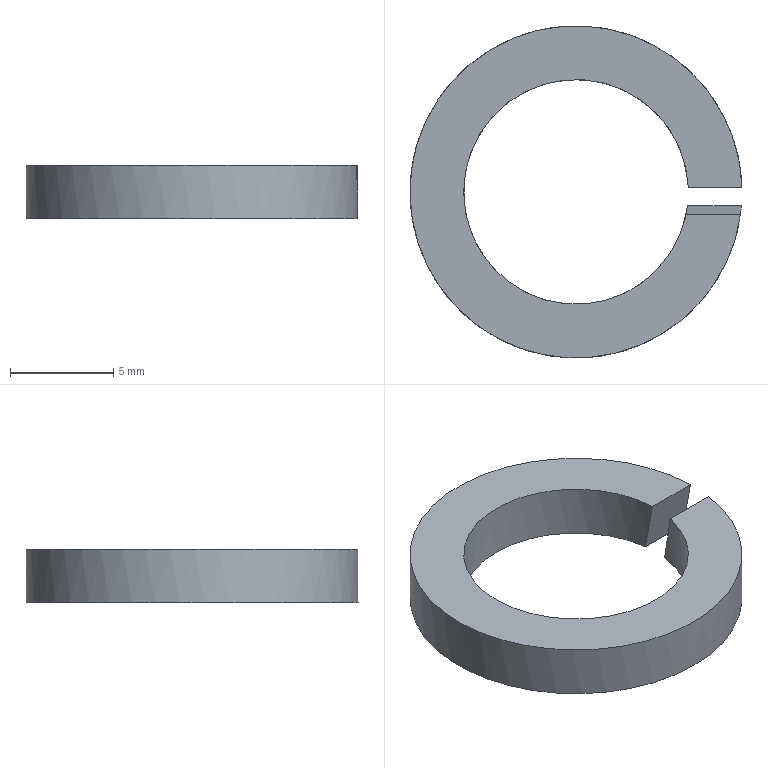Part | NX | 1 solid | 6 faces | box 16.097 x 16.1 x 2.6 mm | volume 277.756 mm3 | plane 4 | cylinder 2 | commonest cylinder face diameters 10.9 x1 16.1 x1
STEP:
#1=CARTESIAN_POINT('',(8.023,-0.66,0.));
#2=VERTEX_POINT('',#1);
#3=CARTESIAN_POINT('',(8.023,0.66,0.));
#4=VERTEX_POINT('',#3);
#5=CARTESIAN_POINT('',(0.,0.,0.));
#6=DIRECTION('',(0.,0.,-1.));
#7=DIRECTION('',(-1.,0.,0.));
#8=AXIS2_PLACEMENT_3D('',#5,#6,#7);
#9=CIRCLE('',#8,8.05);
#10=EDGE_CURVE('',#2,#4,#9,.T.);
#11=ORIENTED_EDGE('',*,*,#10,.F.);
#12=CARTESIAN_POINT('',(7.972,-1.118,2.6));
#13=VERTEX_POINT('',#12);
#14=CARTESIAN_POINT('',(0.,0.,-3.743));
#15=DIRECTION('',(0.,-0.9848,-0.1736));
#16=DIRECTION('',(0.,0.1736,-0.9848));
#17=AXIS2_PLACEMENT_3D('',#14,#15,#16);
#18=ELLIPSE('',#17,46.358,8.05);
#19=EDGE_CURVE('',#2,#13,#18,.T.);
#20=ORIENTED_EDGE('',*,*,#19,.T.);
#21=CARTESIAN_POINT('',(8.047,0.2016,2.6));
#22=VERTEX_POINT('',#21);
#23=CARTESIAN_POINT('',(0.,0.,2.6));
#24=DIRECTION('',(0.,0.,-1.));
#25=DIRECTION('',(-1.,0.,0.));
#26=AXIS2_PLACEMENT_3D('',#23,#24,#25);
#27=CIRCLE('',#26,8.05);
#28=EDGE_CURVE('',#13,#22,#27,.T.);
#29=ORIENTED_EDGE('',*,*,#28,.T.);
#30=CARTESIAN_POINT('',(0.,0.,3.743));
#31=DIRECTION('',(0.,0.9848,0.1736));
#32=DIRECTION('',(0.,0.1736,-0.9848));
#33=AXIS2_PLACEMENT_3D('',#30,#31,#32);
#34=ELLIPSE('',#33,46.358,8.05);
#35=EDGE_CURVE('',#22,#4,#34,.T.);
#36=ORIENTED_EDGE('',*,*,#35,.T.);
#37=EDGE_LOOP('',(#11,#20,#29,#36));
#38=FACE_OUTER_BOUND('',#37,.T.);
#39=CARTESIAN_POINT('',(0.,0.,0.));
#40=DIRECTION('',(0.,0.,-1.));
#41=DIRECTION('',(1.,0.,0.));
#42=AXIS2_PLACEMENT_3D('',#39,#40,#41);
#43=CYLINDRICAL_SURFACE('',#42,8.05);
#44=ADVANCED_FACE('',(#38),#43,.T.);
#45=ORIENTED_EDGE('',*,*,#28,.F.);
#46=CARTESIAN_POINT('',(5.334,-1.118,2.6));
#47=VERTEX_POINT('',#46);
#48=CARTESIAN_POINT('',(0.,-1.118,2.6));
#49=DIRECTION('',(-1.,0.,0.));
#50=VECTOR('',#49,1.);
#51=LINE('',#48,#50);
#52=EDGE_CURVE('',#13,#47,#51,.T.);
#53=ORIENTED_EDGE('',*,*,#52,.T.);
#54=CARTESIAN_POINT('',(5.446,0.2016,2.6));
#55=VERTEX_POINT('',#54);
#56=CARTESIAN_POINT('',(0.,0.,2.6));
#57=DIRECTION('',(0.,0.,-1.));
#58=DIRECTION('',(-1.,0.,0.));
#59=AXIS2_PLACEMENT_3D('',#56,#57,#58);
#60=CIRCLE('',#59,5.45);
#61=EDGE_CURVE('',#47,#55,#60,.T.);
#62=ORIENTED_EDGE('',*,*,#61,.T.);
#63=CARTESIAN_POINT('',(0.,0.2016,2.6));
#64=DIRECTION('',(1.,0.,0.));
#65=VECTOR('',#64,1.);
#66=LINE('',#63,#65);
#67=EDGE_CURVE('',#55,#22,#66,.T.);
#68=ORIENTED_EDGE('',*,*,#67,.T.);
#69=EDGE_LOOP('',(#45,#53,#62,#68));
#70=FACE_OUTER_BOUND('',#69,.T.);
#71=CARTESIAN_POINT('',(0.,8.05,2.6));
#72=DIRECTION('',(0.,0.,1.));
#73=DIRECTION('',(-1.,0.,0.));
#74=AXIS2_PLACEMENT_3D('',#71,#72,#73);
#75=PLANE('',#74);
#76=ADVANCED_FACE('',(#70),#75,.T.);
#77=ORIENTED_EDGE('',*,*,#61,.F.);
#78=CARTESIAN_POINT('',(5.41,-0.66,0.));
#79=VERTEX_POINT('',#78);
#80=CARTESIAN_POINT('',(0.,0.,-3.743));
#81=DIRECTION('',(0.,0.9848,0.1736));
#82=DIRECTION('',(0.,0.1736,-0.9848));
#83=AXIS2_PLACEMENT_3D('',#80,#81,#82);
#84=ELLIPSE('',#83,31.385,5.45);
#85=EDGE_CURVE('',#47,#79,#84,.T.);
#86=ORIENTED_EDGE('',*,*,#85,.T.);
#87=CARTESIAN_POINT('',(5.41,0.66,0.));
#88=VERTEX_POINT('',#87);
#89=CARTESIAN_POINT('',(0.,0.,0.));
#90=DIRECTION('',(0.,0.,-1.));
#91=DIRECTION('',(-1.,0.,0.));
#92=AXIS2_PLACEMENT_3D('',#89,#90,#91);
#93=CIRCLE('',#92,5.45);
#94=EDGE_CURVE('',#79,#88,#93,.T.);
#95=ORIENTED_EDGE('',*,*,#94,.T.);
#96=CARTESIAN_POINT('',(0.,0.,3.743));
#97=DIRECTION('',(0.,-0.9848,-0.1736));
#98=DIRECTION('',(0.,0.1736,-0.9848));
#99=AXIS2_PLACEMENT_3D('',#96,#97,#98);
#100=ELLIPSE('',#99,31.385,5.45);
#101=EDGE_CURVE('',#88,#55,#100,.T.);
#102=ORIENTED_EDGE('',*,*,#101,.T.);
#103=EDGE_LOOP('',(#77,#86,#95,#102));
#104=FACE_OUTER_BOUND('',#103,.T.);
#105=CARTESIAN_POINT('',(0.,0.,0.));
#106=DIRECTION('',(0.,0.,-1.));
#107=DIRECTION('',(1.,0.,0.));
#108=AXIS2_PLACEMENT_3D('',#105,#106,#107);
#109=CYLINDRICAL_SURFACE('',#108,5.45);
#110=ADVANCED_FACE('',(#104),#109,.F.);
#111=ORIENTED_EDGE('',*,*,#94,.F.);
#112=CARTESIAN_POINT('',(0.,-0.66,0.));
#113=DIRECTION('',(1.,0.,0.));
#114=VECTOR('',#113,1.);
#115=LINE('',#112,#114);
#116=EDGE_CURVE('',#79,#2,#115,.T.);
#117=ORIENTED_EDGE('',*,*,#116,.T.);
#118=ORIENTED_EDGE('',*,*,#10,.T.);
#119=CARTESIAN_POINT('',(0.,0.66,0.));
#120=DIRECTION('',(-1.,0.,0.));
#121=VECTOR('',#120,1.);
#122=LINE('',#119,#121);
#123=EDGE_CURVE('',#4,#88,#122,.T.);
#124=ORIENTED_EDGE('',*,*,#123,.T.);
#125=EDGE_LOOP('',(#111,#117,#118,#124));
#126=FACE_OUTER_BOUND('',#125,.T.);
#127=CARTESIAN_POINT('',(0.,5.45,0.));
#128=DIRECTION('',(0.,0.,-1.));
#129=DIRECTION('',(1.,0.,0.));
#130=AXIS2_PLACEMENT_3D('',#127,#128,#129);
#131=PLANE('',#130);
#132=ADVANCED_FACE('',(#126),#131,.T.);
#133=ORIENTED_EDGE('',*,*,#67,.F.);
#134=ORIENTED_EDGE('',*,*,#101,.F.);
#135=ORIENTED_EDGE('',*,*,#123,.F.);
#136=ORIENTED_EDGE('',*,*,#35,.F.);
#137=EDGE_LOOP('',(#133,#134,#135,#136));
#138=FACE_OUTER_BOUND('',#137,.T.);
#139=CARTESIAN_POINT('',(12.075,1.317,-3.728));
#140=DIRECTION('',(0.,-0.9848,-0.1736));
#141=DIRECTION('',(0.,-0.1736,0.9848));
#142=AXIS2_PLACEMENT_3D('',#139,#140,#141);
#143=PLANE('',#142);
#144=ADVANCED_FACE('',(#138),#143,.T.);
#145=ORIENTED_EDGE('',*,*,#116,.F.);
#146=ORIENTED_EDGE('',*,*,#85,.F.);
#147=ORIENTED_EDGE('',*,*,#52,.F.);
#148=ORIENTED_EDGE('',*,*,#19,.F.);
#149=EDGE_LOOP('',(#145,#146,#147,#148));
#150=FACE_OUTER_BOUND('',#149,.T.);
#151=CARTESIAN_POINT('',(12.075,-1.317,3.728));
#152=DIRECTION('',(0.,0.9848,0.1736));
#153=DIRECTION('',(0.,0.1736,-0.9848));
#154=AXIS2_PLACEMENT_3D('',#151,#152,#153);
#155=PLANE('',#154);
#156=ADVANCED_FACE('',(#150),#155,.T.);
#157=CLOSED_SHELL('',(#44,#76,#110,#132,#144,#156));
#158=MANIFOLD_SOLID_BREP('',#157);
#159=(LENGTH_UNIT()NAMED_UNIT(*)SI_UNIT(.MILLI.,.METRE.));
#160=UNCERTAINTY_MEASURE_WITH_UNIT(LENGTH_MEASURE(0.00002),#159,'','');
#161=(NAMED_UNIT(*)PLANE_ANGLE_UNIT()SI_UNIT($,.RADIAN.));
#162=PLANE_ANGLE_MEASURE_WITH_UNIT(PLANE_ANGLE_MEASURE(0.01745),#161);
#163=DIMENSIONAL_EXPONENTS(0.,0.,0.,0.,0.,0.,0.);
#164=(CONVERSION_BASED_UNIT('DEGREE',#162)NAMED_UNIT(#163)PLANE_ANGLE_UNIT());
#165=(NAMED_UNIT(*)SI_UNIT($,.STERADIAN.)SOLID_ANGLE_UNIT());
#166=(GEOMETRIC_REPRESENTATION_CONTEXT(3)GLOBAL_UNCERTAINTY_ASSIGNED_CONTEXT((#160))GLOBAL_UNIT_ASSIGNED_CONTEXT((#159,#164,#165))REPRESENTATION_CONTEXT('',''));
#167=ADVANCED_BREP_SHAPE_REPRESENTATION('',(#158),#166);